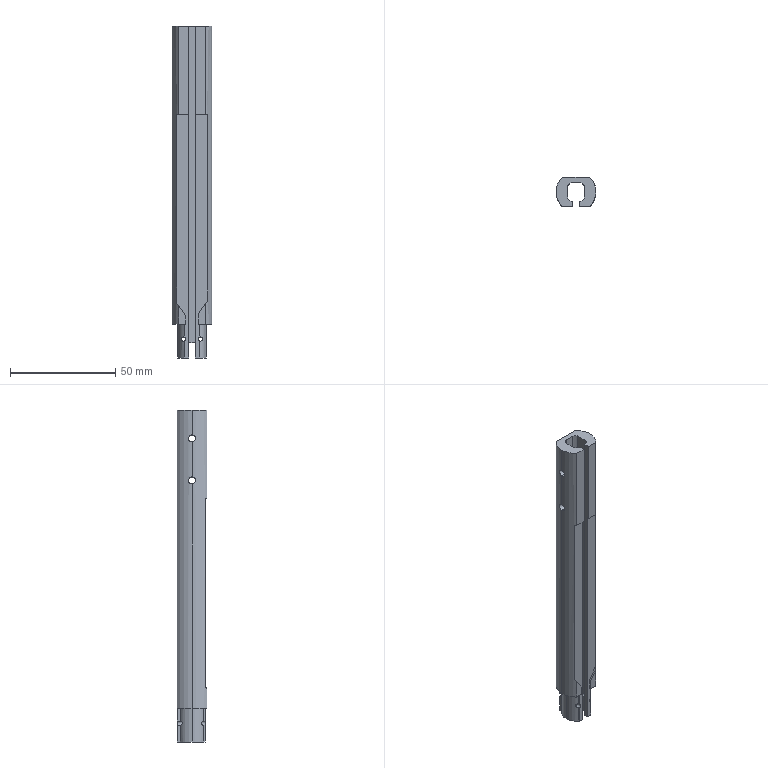Part | STEP file | magnetic tile top shaft | 1 solid | 62 faces | box 19 x 14 x 158 mm | volume 23396 mm3 | plane 38 | cylinder 24 | commonest cylinder face diameters 3.3 x8 2 x6 10 x4 13.4 x3 19 x3